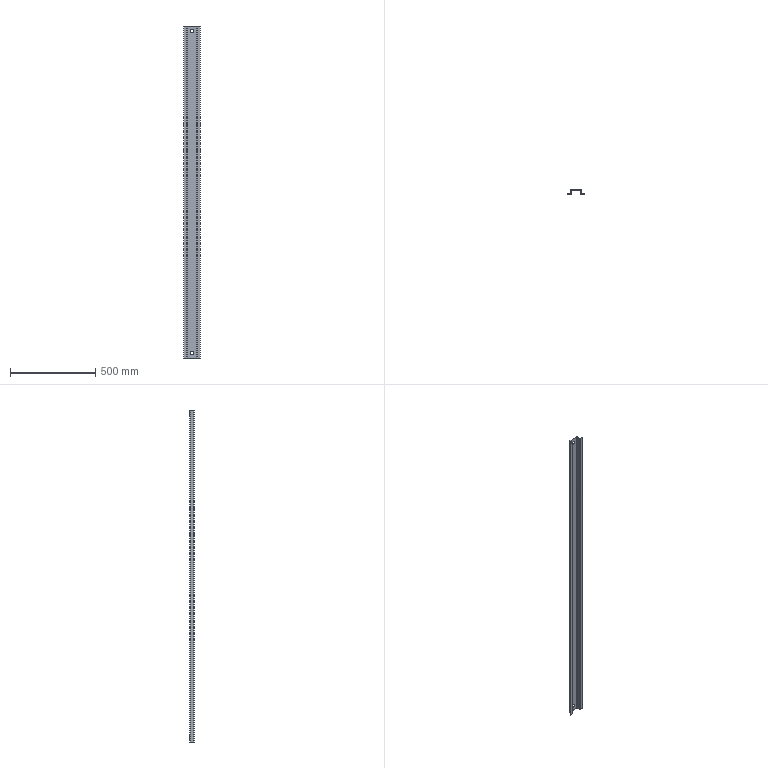Part | 1 solid | 42 faces | box 98.4 x 25 x 1951 mm | volume 224871 mm3 | plane 30 | cylinder 12 | commonest cylinder face diameters 2 x4 3.6 x4 20 x4
STEP:
#1=CARTESIAN_POINT('',(10.,-0.8,945.5));
#2=VERTEX_POINT('',#1);
#3=CARTESIAN_POINT('',(-10.,-0.8,945.5));
#4=VERTEX_POINT('',#3);
#5=CARTESIAN_POINT('',(0.,-0.8,945.5));
#6=DIRECTION('',(0.,1.,0.));
#7=DIRECTION('',(-1.,0.,0.));
#8=AXIS2_PLACEMENT_3D('',#5,#6,#7);
#9=CIRCLE('',#8,10.);
#10=EDGE_CURVE('',#2,#4,#9,.T.);
#11=ORIENTED_EDGE('',*,*,#10,.F.);
#12=CARTESIAN_POINT('',(10.,0.,945.5));
#13=VERTEX_POINT('',#12);
#14=CARTESIAN_POINT('',(10.,-10.,945.5));
#15=DIRECTION('',(0.,1.,0.));
#16=VECTOR('',#15,1000.);
#17=LINE('',#14,#16);
#18=EDGE_CURVE('',#2,#13,#17,.T.);
#19=ORIENTED_EDGE('',*,*,#18,.T.);
#20=CARTESIAN_POINT('',(-10.,0.,945.5));
#21=VERTEX_POINT('',#20);
#22=CARTESIAN_POINT('',(0.,0.,945.5));
#23=DIRECTION('',(0.,1.,0.));
#24=DIRECTION('',(-1.,0.,0.));
#25=AXIS2_PLACEMENT_3D('',#22,#23,#24);
#26=CIRCLE('',#25,10.);
#27=EDGE_CURVE('',#13,#21,#26,.T.);
#28=ORIENTED_EDGE('',*,*,#27,.T.);
#29=CARTESIAN_POINT('',(-10.,-10.,945.5));
#30=DIRECTION('',(0.,1.,0.));
#31=VECTOR('',#30,1000.);
#32=LINE('',#29,#31);
#33=EDGE_CURVE('',#4,#21,#32,.T.);
#34=ORIENTED_EDGE('',*,*,#33,.F.);
#35=EDGE_LOOP('',(#11,#19,#28,#34));
#36=FACE_OUTER_BOUND('',#35,.T.);
#37=CARTESIAN_POINT('',(0.,-10.,945.5));
#38=DIRECTION('',(0.,1.,0.));
#39=DIRECTION('',(-1.,0.,0.));
#40=AXIS2_PLACEMENT_3D('',#37,#38,#39);
#41=CYLINDRICAL_SURFACE('',#40,10.);
#42=ADVANCED_FACE('',(#36),#41,.F.);
#43=CARTESIAN_POINT('',(10.,-0.8,-945.5));
#44=VERTEX_POINT('',#43);
#45=CARTESIAN_POINT('',(-10.,-0.8,-945.5));
#46=VERTEX_POINT('',#45);
#47=CARTESIAN_POINT('',(0.,-0.8,-945.5));
#48=DIRECTION('',(0.,1.,0.));
#49=DIRECTION('',(-1.,0.,0.));
#50=AXIS2_PLACEMENT_3D('',#47,#48,#49);
#51=CIRCLE('',#50,10.);
#52=EDGE_CURVE('',#44,#46,#51,.T.);
#53=ORIENTED_EDGE('',*,*,#52,.F.);
#54=CARTESIAN_POINT('',(10.,0.,-945.5));
#55=VERTEX_POINT('',#54);
#56=CARTESIAN_POINT('',(10.,-10.,-945.5));
#57=DIRECTION('',(0.,1.,0.));
#58=VECTOR('',#57,1000.);
#59=LINE('',#56,#58);
#60=EDGE_CURVE('',#44,#55,#59,.T.);
#61=ORIENTED_EDGE('',*,*,#60,.T.);
#62=CARTESIAN_POINT('',(-10.,0.,-945.5));
#63=VERTEX_POINT('',#62);
#64=CARTESIAN_POINT('',(0.,0.,-945.5));
#65=DIRECTION('',(0.,1.,0.));
#66=DIRECTION('',(1.,0.,0.));
#67=AXIS2_PLACEMENT_3D('',#64,#65,#66);
#68=CIRCLE('',#67,10.);
#69=EDGE_CURVE('',#55,#63,#68,.T.);
#70=ORIENTED_EDGE('',*,*,#69,.T.);
#71=CARTESIAN_POINT('',(-10.,-10.,-945.5));
#72=DIRECTION('',(0.,1.,0.));
#73=VECTOR('',#72,1000.);
#74=LINE('',#71,#73);
#75=EDGE_CURVE('',#46,#63,#74,.T.);
#76=ORIENTED_EDGE('',*,*,#75,.F.);
#77=EDGE_LOOP('',(#53,#61,#70,#76));
#78=FACE_OUTER_BOUND('',#77,.T.);
#79=CARTESIAN_POINT('',(0.,-10.,-945.5));
#80=DIRECTION('',(0.,1.,0.));
#81=DIRECTION('',(-1.,0.,0.));
#82=AXIS2_PLACEMENT_3D('',#79,#80,#81);
#83=CYLINDRICAL_SURFACE('',#82,10.);
#84=ADVANCED_FACE('',(#78),#83,.F.);
#85=CARTESIAN_POINT('',(29.2,-23.2,-975.5));
#86=VERTEX_POINT('',#85);
#87=CARTESIAN_POINT('',(29.2,-23.2,975.5));
#88=VERTEX_POINT('',#87);
#89=CARTESIAN_POINT('',(29.2,-23.2,-975.5));
#90=DIRECTION('',(0.,0.,1.));
#91=VECTOR('',#90,1000.);
#92=LINE('',#89,#91);
#93=EDGE_CURVE('',#86,#88,#92,.T.);
#94=ORIENTED_EDGE('',*,*,#93,.T.);
#95=CARTESIAN_POINT('',(29.2,-1.8,975.5));
#96=VERTEX_POINT('',#95);
#97=CARTESIAN_POINT('',(29.2,0.,975.5));
#98=DIRECTION('',(0.,-1.,0.));
#99=VECTOR('',#98,1000.);
#100=LINE('',#97,#99);
#101=EDGE_CURVE('',#96,#88,#100,.T.);
#102=ORIENTED_EDGE('',*,*,#101,.F.);
#103=CARTESIAN_POINT('',(29.2,-1.8,-975.5));
#104=VERTEX_POINT('',#103);
#105=CARTESIAN_POINT('',(29.2,-1.8,975.5));
#106=DIRECTION('',(0.,0.,-1.));
#107=VECTOR('',#106,1000.);
#108=LINE('',#105,#107);
#109=EDGE_CURVE('',#96,#104,#108,.T.);
#110=ORIENTED_EDGE('',*,*,#109,.T.);
#111=CARTESIAN_POINT('',(29.2,0.,-975.5));
#112=DIRECTION('',(0.,-1.,0.));
#113=VECTOR('',#112,1000.);
#114=LINE('',#111,#113);
#115=EDGE_CURVE('',#104,#86,#114,.T.);
#116=ORIENTED_EDGE('',*,*,#115,.T.);
#117=EDGE_LOOP('',(#94,#102,#110,#116));
#118=FACE_OUTER_BOUND('',#117,.T.);
#119=CARTESIAN_POINT('',(29.2,0.,975.5));
#120=DIRECTION('',(1.,0.,0.));
#121=DIRECTION('',(0.,1.,0.));
#122=AXIS2_PLACEMENT_3D('',#119,#120,#121);
#123=PLANE('',#122);
#124=ADVANCED_FACE('',(#118),#123,.F.);
#125=CARTESIAN_POINT('',(30.,-1.8,975.5));
#126=VERTEX_POINT('',#125);
#127=CARTESIAN_POINT('',(30.,-23.2,975.5));
#128=VERTEX_POINT('',#127);
#129=CARTESIAN_POINT('',(30.,0.,975.5));
#130=DIRECTION('',(0.,-1.,0.));
#131=VECTOR('',#130,1000.);
#132=LINE('',#129,#131);
#133=EDGE_CURVE('',#126,#128,#132,.T.);
#134=ORIENTED_EDGE('',*,*,#133,.T.);
#135=CARTESIAN_POINT('',(30.,-23.2,-975.5));
#136=VERTEX_POINT('',#135);
#137=CARTESIAN_POINT('',(30.,-23.2,-975.5));
#138=DIRECTION('',(0.,0.,1.));
#139=VECTOR('',#138,1000.);
#140=LINE('',#137,#139);
#141=EDGE_CURVE('',#136,#128,#140,.T.);
#142=ORIENTED_EDGE('',*,*,#141,.F.);
#143=CARTESIAN_POINT('',(30.,-1.8,-975.5));
#144=VERTEX_POINT('',#143);
#145=CARTESIAN_POINT('',(30.,0.,-975.5));
#146=DIRECTION('',(0.,-1.,0.));
#147=VECTOR('',#146,1000.);
#148=LINE('',#145,#147);
#149=EDGE_CURVE('',#144,#136,#148,.T.);
#150=ORIENTED_EDGE('',*,*,#149,.F.);
#151=CARTESIAN_POINT('',(30.,-1.8,975.5));
#152=DIRECTION('',(0.,0.,-1.));
#153=VECTOR('',#152,1000.);
#154=LINE('',#151,#153);
#155=EDGE_CURVE('',#126,#144,#154,.T.);
#156=ORIENTED_EDGE('',*,*,#155,.F.);
#157=EDGE_LOOP('',(#134,#142,#150,#156));
#158=FACE_OUTER_BOUND('',#157,.T.);
#159=CARTESIAN_POINT('',(30.,0.,975.5));
#160=DIRECTION('',(1.,0.,0.));
#161=DIRECTION('',(0.,1.,0.));
#162=AXIS2_PLACEMENT_3D('',#159,#160,#161);
#163=PLANE('',#162);
#164=ADVANCED_FACE('',(#158),#163,.T.);
#165=CARTESIAN_POINT('',(30.,-23.2,-975.5));
#166=DIRECTION('',(-1.,0.,0.));
#167=VECTOR('',#166,1000.);
#168=LINE('',#165,#167);
#169=EDGE_CURVE('',#136,#86,#168,.T.);
#170=ORIENTED_EDGE('',*,*,#169,.T.);
#171=ORIENTED_EDGE('',*,*,#115,.F.);
#172=CARTESIAN_POINT('',(29.2,-1.8,-975.5));
#173=DIRECTION('',(1.,0.,0.));
#174=VECTOR('',#173,1000.);
#175=LINE('',#172,#174);
#176=EDGE_CURVE('',#104,#144,#175,.T.);
#177=ORIENTED_EDGE('',*,*,#176,.T.);
#178=ORIENTED_EDGE('',*,*,#149,.T.);
#179=EDGE_LOOP('',(#170,#171,#177,#178));
#180=FACE_OUTER_BOUND('',#179,.T.);
#181=CARTESIAN_POINT('',(28.2,-1.8,-975.5));
#182=DIRECTION('',(0.,0.,1.));
#183=DIRECTION('',(1.,0.,0.));
#184=AXIS2_PLACEMENT_3D('',#181,#182,#183);
#185=PLANE('',#184);
#186=ADVANCED_FACE('',(#180),#185,.F.);
#187=CARTESIAN_POINT('',(-30.,-23.2,-975.5));
#188=VERTEX_POINT('',#187);
#189=CARTESIAN_POINT('',(-30.,-1.8,-975.5));
#190=VERTEX_POINT('',#189);
#191=CARTESIAN_POINT('',(-30.,-25.,-975.5));
#192=DIRECTION('',(0.,1.,0.));
#193=VECTOR('',#192,1000.);
#194=LINE('',#191,#193);
#195=EDGE_CURVE('',#188,#190,#194,.T.);
#196=ORIENTED_EDGE('',*,*,#195,.F.);
#197=CARTESIAN_POINT('',(-30.,-23.2,975.5));
#198=VERTEX_POINT('',#197);
#199=CARTESIAN_POINT('',(-30.,-23.2,975.5));
#200=DIRECTION('',(0.,0.,-1.));
#201=VECTOR('',#200,1000.);
#202=LINE('',#199,#201);
#203=EDGE_CURVE('',#198,#188,#202,.T.);
#204=ORIENTED_EDGE('',*,*,#203,.F.);
#205=CARTESIAN_POINT('',(-30.,-1.8,975.5));
#206=VERTEX_POINT('',#205);
#207=CARTESIAN_POINT('',(-30.,-25.,975.5));
#208=DIRECTION('',(0.,1.,0.));
#209=VECTOR('',#208,1000.);
#210=LINE('',#207,#209);
#211=EDGE_CURVE('',#198,#206,#210,.T.);
#212=ORIENTED_EDGE('',*,*,#211,.T.);
#213=CARTESIAN_POINT('',(-30.,-1.8,975.5));
#214=DIRECTION('',(0.,0.,-1.));
#215=VECTOR('',#214,1000.);
#216=LINE('',#213,#215);
#217=EDGE_CURVE('',#206,#190,#216,.T.);
#218=ORIENTED_EDGE('',*,*,#217,.T.);
#219=EDGE_LOOP('',(#196,#204,#212,#218));
#220=FACE_OUTER_BOUND('',#219,.T.);
#221=CARTESIAN_POINT('',(-30.,-25.,975.5));
#222=DIRECTION('',(-1.,0.,0.));
#223=DIRECTION('',(0.,0.,1.));
#224=AXIS2_PLACEMENT_3D('',#221,#222,#223);
#225=PLANE('',#224);
#226=ADVANCED_FACE('',(#220),#225,.T.);
#227=CARTESIAN_POINT('',(-29.2,-23.2,975.5));
#228=VERTEX_POINT('',#227);
#229=CARTESIAN_POINT('',(-29.2,-23.2,-975.5));
#230=VERTEX_POINT('',#229);
#231=CARTESIAN_POINT('',(-29.2,-23.2,975.5));
#232=DIRECTION('',(0.,0.,-1.));
#233=VECTOR('',#232,1000.);
#234=LINE('',#231,#233);
#235=EDGE_CURVE('',#228,#230,#234,.T.);
#236=ORIENTED_EDGE('',*,*,#235,.T.);
#237=CARTESIAN_POINT('',(-29.2,-1.8,-975.5));
#238=VERTEX_POINT('',#237);
#239=CARTESIAN_POINT('',(-29.2,-25.,-975.5));
#240=DIRECTION('',(0.,1.,0.));
#241=VECTOR('',#240,1000.);
#242=LINE('',#239,#241);
#243=EDGE_CURVE('',#230,#238,#242,.T.);
#244=ORIENTED_EDGE('',*,*,#243,.T.);
#245=CARTESIAN_POINT('',(-29.2,-1.8,975.5));
#246=VERTEX_POINT('',#245);
#247=CARTESIAN_POINT('',(-29.2,-1.8,975.5));
#248=DIRECTION('',(0.,0.,-1.));
#249=VECTOR('',#248,1000.);
#250=LINE('',#247,#249);
#251=EDGE_CURVE('',#246,#238,#250,.T.);
#252=ORIENTED_EDGE('',*,*,#251,.F.);
#253=CARTESIAN_POINT('',(-29.2,-25.,975.5));
#254=DIRECTION('',(0.,1.,0.));
#255=VECTOR('',#254,1000.);
#256=LINE('',#253,#255);
#257=EDGE_CURVE('',#228,#246,#256,.T.);
#258=ORIENTED_EDGE('',*,*,#257,.F.);
#259=EDGE_LOOP('',(#236,#244,#252,#258));
#260=FACE_OUTER_BOUND('',#259,.T.);
#261=CARTESIAN_POINT('',(-29.2,-25.,975.5));
#262=DIRECTION('',(-1.,0.,0.));
#263=DIRECTION('',(0.,0.,1.));
#264=AXIS2_PLACEMENT_3D('',#261,#262,#263);
#265=PLANE('',#264);
#266=ADVANCED_FACE('',(#260),#265,.F.);
#267=ORIENTED_EDGE('',*,*,#211,.F.);
#268=CARTESIAN_POINT('',(-30.,-23.2,975.5));
#269=DIRECTION('',(1.,0.,0.));
#270=VECTOR('',#269,1000.);
#271=LINE('',#268,#270);
#272=EDGE_CURVE('',#198,#228,#271,.T.);
#273=ORIENTED_EDGE('',*,*,#272,.T.);
#274=ORIENTED_EDGE('',*,*,#257,.T.);
#275=CARTESIAN_POINT('',(-29.2,-1.8,975.5));
#276=DIRECTION('',(-1.,0.,0.));
#277=VECTOR('',#276,1000.);
#278=LINE('',#275,#277);
#279=EDGE_CURVE('',#246,#206,#278,.T.);
#280=ORIENTED_EDGE('',*,*,#279,.T.);
#281=EDGE_LOOP('',(#267,#273,#274,#280));
#282=FACE_OUTER_BOUND('',#281,.T.);
#283=CARTESIAN_POINT('',(28.2,-1.8,975.5));
#284=DIRECTION('',(0.,0.,1.));
#285=DIRECTION('',(1.,0.,0.));
#286=AXIS2_PLACEMENT_3D('',#283,#284,#285);
#287=PLANE('',#286);
#288=ADVANCED_FACE('',(#282),#287,.T.);
#289=CARTESIAN_POINT('',(-28.2,0.,975.5));
#290=VERTEX_POINT('',#289);
#291=CARTESIAN_POINT('',(-28.2,-0.8,975.5));
#292=VERTEX_POINT('',#291);
#293=CARTESIAN_POINT('',(-28.2,0.,975.5));
#294=DIRECTION('',(0.,-1.,0.));
#295=VECTOR('',#294,1000.);
#296=LINE('',#293,#295);
#297=EDGE_CURVE('',#290,#292,#296,.T.);
#298=ORIENTED_EDGE('',*,*,#297,.F.);
#299=CARTESIAN_POINT('',(-28.2,-1.8,975.5));
#300=DIRECTION('',(0.,0.,-1.));
#301=DIRECTION('',(1.,0.,0.));
#302=AXIS2_PLACEMENT_3D('',#299,#300,#301);
#303=CIRCLE('',#302,1.8);
#304=EDGE_CURVE('',#206,#290,#303,.T.);
#305=ORIENTED_EDGE('',*,*,#304,.F.);
#306=ORIENTED_EDGE('',*,*,#279,.F.);
#307=CARTESIAN_POINT('',(-28.2,-1.8,975.5));
#308=DIRECTION('',(0.,0.,-1.));
#309=DIRECTION('',(1.,0.,0.));
#310=AXIS2_PLACEMENT_3D('',#307,#308,#309);
#311=CIRCLE('',#310,1.);
#312=EDGE_CURVE('',#246,#292,#311,.T.);
#313=ORIENTED_EDGE('',*,*,#312,.T.);
#314=EDGE_LOOP('',(#298,#305,#306,#313));
#315=FACE_OUTER_BOUND('',#314,.T.);
#316=CARTESIAN_POINT('',(-28.2,0.,975.5));
#317=DIRECTION('',(0.,0.,1.));
#318=DIRECTION('',(1.,0.,0.));
#319=AXIS2_PLACEMENT_3D('',#316,#317,#318);
#320=PLANE('',#319);
#321=ADVANCED_FACE('',(#315),#320,.T.);
#322=CARTESIAN_POINT('',(28.2,0.,975.5));
#323=VERTEX_POINT('',#322);
#324=CARTESIAN_POINT('',(-30.,0.,975.5));
#325=DIRECTION('',(1.,0.,0.));
#326=VECTOR('',#325,1000.);
#327=LINE('',#324,#326);
#328=EDGE_CURVE('',#290,#323,#327,.T.);
#329=ORIENTED_EDGE('',*,*,#328,.F.);
#330=ORIENTED_EDGE('',*,*,#297,.T.);
#331=CARTESIAN_POINT('',(28.2,-0.8,975.5));
#332=VERTEX_POINT('',#331);
#333=CARTESIAN_POINT('',(-30.,-0.8,975.5));
#334=DIRECTION('',(1.,0.,0.));
#335=VECTOR('',#334,1000.);
#336=LINE('',#333,#335);
#337=EDGE_CURVE('',#292,#332,#336,.T.);
#338=ORIENTED_EDGE('',*,*,#337,.T.);
#339=CARTESIAN_POINT('',(28.2,-0.8,975.5));
#340=DIRECTION('',(0.,1.,0.));
#341=VECTOR('',#340,1000.);
#342=LINE('',#339,#341);
#343=EDGE_CURVE('',#332,#323,#342,.T.);
#344=ORIENTED_EDGE('',*,*,#343,.T.);
#345=EDGE_LOOP('',(#329,#330,#338,#344));
#346=FACE_OUTER_BOUND('',#345,.T.);
#347=CARTESIAN_POINT('',(-29.2,-1.8,975.5));
#348=DIRECTION('',(0.,0.,1.));
#349=DIRECTION('',(1.,0.,0.));
#350=AXIS2_PLACEMENT_3D('',#347,#348,#349);
#351=PLANE('',#350);
#352=ADVANCED_FACE('',(#346),#351,.T.);
#353=CARTESIAN_POINT('',(-30.,-1.8,-975.5));
#354=DIRECTION('',(1.,0.,0.));
#355=VECTOR('',#354,1000.);
#356=LINE('',#353,#355);
#357=EDGE_CURVE('',#190,#238,#356,.T.);
#358=ORIENTED_EDGE('',*,*,#357,.F.);
#359=CARTESIAN_POINT('',(-28.2,0.,-975.5));
#360=VERTEX_POINT('',#359);
#361=CARTESIAN_POINT('',(-28.2,-1.8,-975.5));
#362=DIRECTION('',(0.,0.,-1.));
#363=DIRECTION('',(1.,0.,0.));
#364=AXIS2_PLACEMENT_3D('',#361,#362,#363);
#365=CIRCLE('',#364,1.8);
#366=EDGE_CURVE('',#190,#360,#365,.T.);
#367=ORIENTED_EDGE('',*,*,#366,.T.);
#368=CARTESIAN_POINT('',(-28.2,-0.8,-975.5));
#369=VERTEX_POINT('',#368);
#370=CARTESIAN_POINT('',(-28.2,-0.8,-975.5));
#371=DIRECTION('',(0.,1.,0.));
#372=VECTOR('',#371,1000.);
#373=LINE('',#370,#372);
#374=EDGE_CURVE('',#369,#360,#373,.T.);
#375=ORIENTED_EDGE('',*,*,#374,.F.);
#376=CARTESIAN_POINT('',(-28.2,-1.8,-975.5));
#377=DIRECTION('',(0.,0.,-1.));
#378=DIRECTION('',(1.,0.,0.));
#379=AXIS2_PLACEMENT_3D('',#376,#377,#378);
#380=CIRCLE('',#379,1.);
#381=EDGE_CURVE('',#238,#369,#380,.T.);
#382=ORIENTED_EDGE('',*,*,#381,.F.);
#383=EDGE_LOOP('',(#358,#367,#375,#382));
#384=FACE_OUTER_BOUND('',#383,.T.);
#385=CARTESIAN_POINT('',(-30.,-1.8,-975.5));
#386=DIRECTION('',(0.,0.,-1.));
#387=DIRECTION('',(-1.,0.,0.));
#388=AXIS2_PLACEMENT_3D('',#385,#386,#387);
#389=PLANE('',#388);
#390=ADVANCED_FACE('',(#384),#389,.T.);
#391=CARTESIAN_POINT('',(-30.,-23.2,-975.5));
#392=DIRECTION('',(1.,0.,0.));
#393=VECTOR('',#392,1000.);
#394=LINE('',#391,#393);
#395=EDGE_CURVE('',#188,#230,#394,.T.);
#396=ORIENTED_EDGE('',*,*,#395,.F.);
#397=ORIENTED_EDGE('',*,*,#195,.T.);
#398=ORIENTED_EDGE('',*,*,#357,.T.);
#399=ORIENTED_EDGE('',*,*,#243,.F.);
#400=EDGE_LOOP('',(#396,#397,#398,#399));
#401=FACE_OUTER_BOUND('',#400,.T.);
#402=CARTESIAN_POINT('',(-28.2,-0.8,-975.5));
#403=DIRECTION('',(0.,0.,-1.));
#404=DIRECTION('',(-1.,0.,0.));
#405=AXIS2_PLACEMENT_3D('',#402,#403,#404);
#406=PLANE('',#405);
#407=ADVANCED_FACE('',(#401),#406,.T.);
#408=CARTESIAN_POINT('',(30.,-1.8,975.5));
#409=DIRECTION('',(-1.,0.,0.));
#410=VECTOR('',#409,1000.);
#411=LINE('',#408,#410);
#412=EDGE_CURVE('',#126,#96,#411,.T.);
#413=ORIENTED_EDGE('',*,*,#412,.F.);
#414=CARTESIAN_POINT('',(28.2,-1.8,975.5));
#415=DIRECTION('',(0.,0.,-1.));
#416=DIRECTION('',(1.,0.,0.));
#417=AXIS2_PLACEMENT_3D('',#414,#415,#416);
#418=CIRCLE('',#417,1.8);
#419=EDGE_CURVE('',#323,#126,#418,.T.);
#420=ORIENTED_EDGE('',*,*,#419,.F.);
#421=ORIENTED_EDGE('',*,*,#343,.F.);
#422=CARTESIAN_POINT('',(28.2,-1.8,975.5));
#423=DIRECTION('',(0.,0.,-1.));
#424=DIRECTION('',(1.,0.,0.));
#425=AXIS2_PLACEMENT_3D('',#422,#423,#424);
#426=CIRCLE('',#425,1.);
#427=EDGE_CURVE('',#332,#96,#426,.T.);
#428=ORIENTED_EDGE('',*,*,#427,.T.);
#429=EDGE_LOOP('',(#413,#420,#421,#428));
#430=FACE_OUTER_BOUND('',#429,.T.);
#431=CARTESIAN_POINT('',(30.,-1.8,975.5));
#432=DIRECTION('',(0.,0.,1.));
#433=DIRECTION('',(1.,0.,0.));
#434=AXIS2_PLACEMENT_3D('',#431,#432,#433);
#435=PLANE('',#434);
#436=ADVANCED_FACE('',(#430),#435,.T.);
#437=CARTESIAN_POINT('',(30.,-23.2,975.5));
#438=DIRECTION('',(-1.,0.,0.));
#439=VECTOR('',#438,1000.);
#440=LINE('',#437,#439);
#441=EDGE_CURVE('',#128,#88,#440,.T.);
#442=ORIENTED_EDGE('',*,*,#441,.F.);
#443=ORIENTED_EDGE('',*,*,#133,.F.);
#444=ORIENTED_EDGE('',*,*,#412,.T.);
#445=ORIENTED_EDGE('',*,*,#101,.T.);
#446=EDGE_LOOP('',(#442,#443,#444,#445));
#447=FACE_OUTER_BOUND('',#446,.T.);
#448=CARTESIAN_POINT('',(28.2,-0.8,975.5));
#449=DIRECTION('',(0.,0.,1.));
#450=DIRECTION('',(1.,0.,0.));
#451=AXIS2_PLACEMENT_3D('',#448,#449,#450);
#452=PLANE('',#451);
#453=ADVANCED_FACE('',(#447),#452,.T.);
#454=CARTESIAN_POINT('',(28.2,0.,-975.5));
#455=VERTEX_POINT('',#454);
#456=CARTESIAN_POINT('',(28.2,-0.8,-975.5));
#457=VERTEX_POINT('',#456);
#458=CARTESIAN_POINT('',(28.2,0.,-975.5));
#459=DIRECTION('',(0.,-1.,0.));
#460=VECTOR('',#459,1000.);
#461=LINE('',#458,#460);
#462=EDGE_CURVE('',#455,#457,#461,.T.);
#463=ORIENTED_EDGE('',*,*,#462,.F.);
#464=CARTESIAN_POINT('',(28.2,-1.8,-975.5));
#465=DIRECTION('',(0.,0.,-1.));
#466=DIRECTION('',(1.,0.,0.));
#467=AXIS2_PLACEMENT_3D('',#464,#465,#466);
#468=CIRCLE('',#467,1.8);
#469=EDGE_CURVE('',#455,#144,#468,.T.);
#470=ORIENTED_EDGE('',*,*,#469,.T.);
#471=ORIENTED_EDGE('',*,*,#176,.F.);
#472=CARTESIAN_POINT('',(28.2,-1.8,-975.5));
#473=DIRECTION('',(0.,0.,-1.));
#474=DIRECTION('',(1.,0.,0.));
#475=AXIS2_PLACEMENT_3D('',#472,#473,#474);
#476=CIRCLE('',#475,1.);
#477=EDGE_CURVE('',#457,#104,#476,.T.);
#478=ORIENTED_EDGE('',*,*,#477,.F.);
#479=EDGE_LOOP('',(#463,#470,#471,#478));
#480=FACE_OUTER_BOUND('',#479,.T.);
#481=CARTESIAN_POINT('',(28.2,0.,-975.5));
#482=DIRECTION('',(0.,0.,-1.));
#483=DIRECTION('',(-1.,0.,0.));
#484=AXIS2_PLACEMENT_3D('',#481,#482,#483);
#485=PLANE('',#484);
#486=ADVANCED_FACE('',(#480),#485,.T.);
#487=CARTESIAN_POINT('',(-30.,0.,-975.5));
#488=DIRECTION('',(1.,0.,0.));
#489=VECTOR('',#488,1000.);
#490=LINE('',#487,#489);
#491=EDGE_CURVE('',#360,#455,#490,.T.);
#492=ORIENTED_EDGE('',*,*,#491,.T.);
#493=ORIENTED_EDGE('',*,*,#462,.T.);
#494=CARTESIAN_POINT('',(-30.,-0.8,-975.5));
#495=DIRECTION('',(1.,0.,0.));
#496=VECTOR('',#495,1000.);
#497=LINE('',#494,#496);
#498=EDGE_CURVE('',#369,#457,#497,.T.);
#499=ORIENTED_EDGE('',*,*,#498,.F.);
#500=ORIENTED_EDGE('',*,*,#374,.T.);
#501=EDGE_LOOP('',(#492,#493,#499,#500));
#502=FACE_OUTER_BOUND('',#501,.T.);
#503=CARTESIAN_POINT('',(29.2,-1.8,-975.5));
#504=DIRECTION('',(0.,0.,-1.));
#505=DIRECTION('',(-1.,0.,0.));
#506=AXIS2_PLACEMENT_3D('',#503,#504,#505);
#507=PLANE('',#506);
#508=ADVANCED_FACE('',(#502),#507,.T.);
#509=ORIENTED_EDGE('',*,*,#469,.F.);
#510=CARTESIAN_POINT('',(28.2,0.,975.5));
#511=DIRECTION('',(0.,0.,-1.));
#512=VECTOR('',#511,1000.);
#513=LINE('',#510,#512);
#514=EDGE_CURVE('',#323,#455,#513,.T.);
#515=ORIENTED_EDGE('',*,*,#514,.F.);
#516=ORIENTED_EDGE('',*,*,#419,.T.);
#517=ORIENTED_EDGE('',*,*,#155,.T.);
#518=EDGE_LOOP('',(#509,#515,#516,#517));
#519=FACE_OUTER_BOUND('',#518,.T.);
#520=CARTESIAN_POINT('',(28.2,-1.8,975.5));
#521=DIRECTION('',(0.,0.,-1.));
#522=DIRECTION('',(-1.,0.,0.));
#523=AXIS2_PLACEMENT_3D('',#520,#521,#522);
#524=CYLINDRICAL_SURFACE('',#523,1.8);
#525=ADVANCED_FACE('',(#519),#524,.T.);
#526=CARTESIAN_POINT('',(0.,0.,945.5));
#527=DIRECTION('',(0.,1.,0.));
#528=DIRECTION('',(-1.,0.,0.));
#529=AXIS2_PLACEMENT_3D('',#526,#527,#528);
#530=CIRCLE('',#529,10.);
#531=EDGE_CURVE('',#21,#13,#530,.T.);
#532=ORIENTED_EDGE('',*,*,#531,.F.);
#533=ORIENTED_EDGE('',*,*,#27,.F.);
#534=EDGE_LOOP('',(#532,#533));
#535=FACE_BOUND('',#534,.T.);
#536=CARTESIAN_POINT('',(0.,0.,-945.5));
#537=DIRECTION('',(0.,1.,0.));
#538=DIRECTION('',(1.,0.,0.));
#539=AXIS2_PLACEMENT_3D('',#536,#537,#538);
#540=CIRCLE('',#539,10.);
#541=EDGE_CURVE('',#63,#55,#540,.T.);
#542=ORIENTED_EDGE('',*,*,#541,.F.);
#543=ORIENTED_EDGE('',*,*,#69,.F.);
#544=EDGE_LOOP('',(#542,#543));
#545=FACE_BOUND('',#544,.T.);
#546=ORIENTED_EDGE('',*,*,#491,.F.);
#547=CARTESIAN_POINT('',(-28.2,0.,975.5));
#548=DIRECTION('',(0.,0.,-1.));
#549=VECTOR('',#548,1000.);
#550=LINE('',#547,#549);
#551=EDGE_CURVE('',#290,#360,#550,.T.);
#552=ORIENTED_EDGE('',*,*,#551,.F.);
#553=ORIENTED_EDGE('',*,*,#328,.T.);
#554=ORIENTED_EDGE('',*,*,#514,.T.);
#555=EDGE_LOOP('',(#546,#552,#553,#554));
#556=FACE_OUTER_BOUND('',#555,.T.);
#557=CARTESIAN_POINT('',(-30.,0.,975.5));
#558=DIRECTION('',(0.,1.,0.));
#559=DIRECTION('',(-1.,0.,0.));
#560=AXIS2_PLACEMENT_3D('',#557,#558,#559);
#561=PLANE('',#560);
#562=ADVANCED_FACE('',(#535,#545,#556),#561,.T.);
#563=ORIENTED_EDGE('',*,*,#366,.F.);
#564=ORIENTED_EDGE('',*,*,#217,.F.);
#565=ORIENTED_EDGE('',*,*,#304,.T.);
#566=ORIENTED_EDGE('',*,*,#551,.T.);
#567=EDGE_LOOP('',(#563,#564,#565,#566));
#568=FACE_OUTER_BOUND('',#567,.T.);
#569=CARTESIAN_POINT('',(-28.2,-1.8,975.5));
#570=DIRECTION('',(0.,0.,-1.));
#571=DIRECTION('',(-1.,0.,0.));
#572=AXIS2_PLACEMENT_3D('',#569,#570,#571);
#573=CYLINDRICAL_SURFACE('',#572,1.8);
#574=ADVANCED_FACE('',(#568),#573,.T.);
#575=ORIENTED_EDGE('',*,*,#381,.T.);
#576=CARTESIAN_POINT('',(-28.2,-0.8,975.5));
#577=DIRECTION('',(0.,0.,-1.));
#578=VECTOR('',#577,1000.);
#579=LINE('',#576,#578);
#580=EDGE_CURVE('',#292,#369,#579,.T.);
#581=ORIENTED_EDGE('',*,*,#580,.F.);
#582=ORIENTED_EDGE('',*,*,#312,.F.);
#583=ORIENTED_EDGE('',*,*,#251,.T.);
#584=EDGE_LOOP('',(#575,#581,#582,#583));
#585=FACE_OUTER_BOUND('',#584,.T.);
#586=CARTESIAN_POINT('',(-28.2,-1.8,975.5));
#587=DIRECTION('',(0.,0.,-1.));
#588=DIRECTION('',(-1.,0.,0.));
#589=AXIS2_PLACEMENT_3D('',#586,#587,#588);
#590=CYLINDRICAL_SURFACE('',#589,1.);
#591=ADVANCED_FACE('',(#585),#590,.F.);
#592=CARTESIAN_POINT('',(0.,-0.8,945.5));
#593=DIRECTION('',(0.,1.,0.));
#594=DIRECTION('',(-1.,0.,0.));
#595=AXIS2_PLACEMENT_3D('',#592,#593,#594);
#596=CIRCLE('',#595,10.);
#597=EDGE_CURVE('',#4,#2,#596,.T.);
#598=ORIENTED_EDGE('',*,*,#597,.T.);
#599=ORIENTED_EDGE('',*,*,#10,.T.);
#600=EDGE_LOOP('',(#598,#599));
#601=FACE_BOUND('',#600,.T.);
#602=CARTESIAN_POINT('',(0.,-0.8,-945.5));
#603=DIRECTION('',(0.,1.,0.));
#604=DIRECTION('',(-1.,0.,0.));
#605=AXIS2_PLACEMENT_3D('',#602,#603,#604);
#606=CIRCLE('',#605,10.);
#607=EDGE_CURVE('',#46,#44,#606,.T.);
#608=ORIENTED_EDGE('',*,*,#607,.T.);
#609=ORIENTED_EDGE('',*,*,#52,.T.);
#610=EDGE_LOOP('',(#608,#609));
#611=FACE_BOUND('',#610,.T.);
#612=ORIENTED_EDGE('',*,*,#498,.T.);
#613=CARTESIAN_POINT('',(28.2,-0.8,975.5));
#614=DIRECTION('',(0.,0.,-1.));
#615=VECTOR('',#614,1000.);
#616=LINE('',#613,#615);
#617=EDGE_CURVE('',#332,#457,#616,.T.);
#618=ORIENTED_EDGE('',*,*,#617,.F.);
#619=ORIENTED_EDGE('',*,*,#337,.F.);
#620=ORIENTED_EDGE('',*,*,#580,.T.);
#621=EDGE_LOOP('',(#612,#618,#619,#620));
#622=FACE_OUTER_BOUND('',#621,.T.);
#623=CARTESIAN_POINT('',(-30.,-0.8,975.5));
#624=DIRECTION('',(0.,1.,0.));
#625=DIRECTION('',(-1.,0.,0.));
#626=AXIS2_PLACEMENT_3D('',#623,#624,#625);
#627=PLANE('',#626);
#628=ADVANCED_FACE('',(#601,#611,#622),#627,.F.);
#629=ORIENTED_EDGE('',*,*,#477,.T.);
#630=ORIENTED_EDGE('',*,*,#109,.F.);
#631=ORIENTED_EDGE('',*,*,#427,.F.);
#632=ORIENTED_EDGE('',*,*,#617,.T.);
#633=EDGE_LOOP('',(#629,#630,#631,#632));
#634=FACE_OUTER_BOUND('',#633,.T.);
#635=CARTESIAN_POINT('',(28.2,-1.8,975.5));
#636=DIRECTION('',(0.,0.,-1.));
#637=DIRECTION('',(-1.,0.,0.));
#638=AXIS2_PLACEMENT_3D('',#635,#636,#637);
#639=CYLINDRICAL_SURFACE('',#638,1.);
#640=ADVANCED_FACE('',(#634),#639,.F.);
#641=CARTESIAN_POINT('',(-31.,-24.2,-975.5));
#642=VERTEX_POINT('',#641);
#643=CARTESIAN_POINT('',(-31.,-25.,-975.5));
#644=VERTEX_POINT('',#643);
#645=CARTESIAN_POINT('',(-31.,-25.,-975.5));
#646=DIRECTION('',(0.,-1.,0.));
#647=VECTOR('',#646,1000.);
#648=LINE('',#645,#647);
#649=EDGE_CURVE('',#642,#644,#648,.T.);
#650=ORIENTED_EDGE('',*,*,#649,.F.);
#651=CARTESIAN_POINT('',(-31.,-23.2,-975.5));
#652=DIRECTION('',(0.,0.,-1.));
#653=DIRECTION('',(1.,0.,0.));
#654=AXIS2_PLACEMENT_3D('',#651,#652,#653);
#655=CIRCLE('',#654,1.);
#656=EDGE_CURVE('',#188,#642,#655,.T.);
#657=ORIENTED_EDGE('',*,*,#656,.F.);
#658=ORIENTED_EDGE('',*,*,#395,.T.);
#659=CARTESIAN_POINT('',(-31.,-23.2,-975.5));
#660=DIRECTION('',(0.,0.,-1.));
#661=DIRECTION('',(1.,0.,0.));
#662=AXIS2_PLACEMENT_3D('',#659,#660,#661);
#663=CIRCLE('',#662,1.8);
#664=EDGE_CURVE('',#230,#644,#663,.T.);
#665=ORIENTED_EDGE('',*,*,#664,.T.);
#666=EDGE_LOOP('',(#650,#657,#658,#665));
#667=FACE_OUTER_BOUND('',#666,.T.);
#668=CARTESIAN_POINT('',(-31.,-23.2,-975.5));
#669=DIRECTION('',(0.,0.,-1.));
#670=DIRECTION('',(-1.,0.,0.));
#671=AXIS2_PLACEMENT_3D('',#668,#669,#670);
#672=PLANE('',#671);
#673=ADVANCED_FACE('',(#667),#672,.T.);
#674=CARTESIAN_POINT('',(-31.,-24.2,975.5));
#675=VERTEX_POINT('',#674);
#676=CARTESIAN_POINT('',(-31.,-23.2,975.5));
#677=DIRECTION('',(0.,0.,1.));
#678=DIRECTION('',(1.,0.,0.));
#679=AXIS2_PLACEMENT_3D('',#676,#677,#678);
#680=CIRCLE('',#679,1.);
#681=EDGE_CURVE('',#675,#198,#680,.T.);
#682=ORIENTED_EDGE('',*,*,#681,.F.);
#683=CARTESIAN_POINT('',(-31.,-25.,975.5));
#684=VERTEX_POINT('',#683);
#685=CARTESIAN_POINT('',(-31.,-24.2,975.5));
#686=DIRECTION('',(0.,-1.,0.));
#687=VECTOR('',#686,1000.);
#688=LINE('',#685,#687);
#689=EDGE_CURVE('',#675,#684,#688,.T.);
#690=ORIENTED_EDGE('',*,*,#689,.T.);
#691=CARTESIAN_POINT('',(-31.,-23.2,975.5));
#692=DIRECTION('',(0.,0.,1.));
#693=DIRECTION('',(1.,0.,0.));
#694=AXIS2_PLACEMENT_3D('',#691,#692,#693);
#695=CIRCLE('',#694,1.8);
#696=EDGE_CURVE('',#684,#228,#695,.T.);
#697=ORIENTED_EDGE('',*,*,#696,.T.);
#698=ORIENTED_EDGE('',*,*,#272,.F.);
#699=EDGE_LOOP('',(#682,#690,#697,#698));
#700=FACE_OUTER_BOUND('',#699,.T.);
#701=CARTESIAN_POINT('',(-31.,-23.2,975.5));
#702=DIRECTION('',(0.,0.,-1.));
#703=DIRECTION('',(-1.,0.,0.));
#704=AXIS2_PLACEMENT_3D('',#701,#702,#703);
#705=PLANE('',#704);
#706=ADVANCED_FACE('',(#700),#705,.F.);
#707=ORIENTED_EDGE('',*,*,#235,.F.);
#708=ORIENTED_EDGE('',*,*,#696,.F.);
#709=CARTESIAN_POINT('',(-31.,-25.,-975.5));
#710=DIRECTION('',(0.,0.,-1.));
#711=VECTOR('',#710,1000.);
#712=LINE('',#709,#711);
#713=EDGE_CURVE('',#684,#644,#712,.T.);
#714=ORIENTED_EDGE('',*,*,#713,.T.);
#715=ORIENTED_EDGE('',*,*,#664,.F.);
#716=EDGE_LOOP('',(#707,#708,#714,#715));
#717=FACE_OUTER_BOUND('',#716,.T.);
#718=CARTESIAN_POINT('',(-31.,-23.2,975.5));
#719=DIRECTION('',(0.,0.,1.));
#720=DIRECTION('',(0.,-1.,0.));
#721=AXIS2_PLACEMENT_3D('',#718,#719,#720);
#722=CYLINDRICAL_SURFACE('',#721,1.8);
#723=ADVANCED_FACE('',(#717),#722,.T.);
#724=ORIENTED_EDGE('',*,*,#203,.T.);
#725=ORIENTED_EDGE('',*,*,#656,.T.);
#726=CARTESIAN_POINT('',(-31.,-24.2,-975.5));
#727=DIRECTION('',(0.,0.,1.));
#728=VECTOR('',#727,1000.);
#729=LINE('',#726,#728);
#730=EDGE_CURVE('',#642,#675,#729,.T.);
#731=ORIENTED_EDGE('',*,*,#730,.T.);
#732=ORIENTED_EDGE('',*,*,#681,.T.);
#733=EDGE_LOOP('',(#724,#725,#731,#732));
#734=FACE_OUTER_BOUND('',#733,.T.);
#735=CARTESIAN_POINT('',(-31.,-23.2,975.5));
#736=DIRECTION('',(0.,0.,1.));
#737=DIRECTION('',(0.,-1.,0.));
#738=AXIS2_PLACEMENT_3D('',#735,#736,#737);
#739=CYLINDRICAL_SURFACE('',#738,1.);
#740=ADVANCED_FACE('',(#734),#739,.F.);
#741=ORIENTED_EDGE('',*,*,#689,.F.);
#742=CARTESIAN_POINT('',(-49.2,-24.2,975.5));
#743=VERTEX_POINT('',#742);
#744=CARTESIAN_POINT('',(-49.2,-24.2,975.5));
#745=DIRECTION('',(-1.,0.,0.));
#746=VECTOR('',#745,1000.);
#747=LINE('',#744,#746);
#748=EDGE_CURVE('',#675,#743,#747,.T.);
#749=ORIENTED_EDGE('',*,*,#748,.T.);
#750=CARTESIAN_POINT('',(-49.2,-25.,975.5));
#751=VERTEX_POINT('',#750);
#752=CARTESIAN_POINT('',(-49.2,-25.,975.5));
#753=DIRECTION('',(0.,1.,0.));
#754=VECTOR('',#753,1000.);
#755=LINE('',#752,#754);
#756=EDGE_CURVE('',#751,#743,#755,.T.);
#757=ORIENTED_EDGE('',*,*,#756,.F.);
#758=CARTESIAN_POINT('',(0.,-25.,975.5));
#759=DIRECTION('',(-1.,0.,0.));
#760=VECTOR('',#759,1000.);
#761=LINE('',#758,#760);
#762=EDGE_CURVE('',#684,#751,#761,.T.);
#763=ORIENTED_EDGE('',*,*,#762,.F.);
#764=EDGE_LOOP('',(#741,#749,#757,#763));
#765=FACE_OUTER_BOUND('',#764,.T.);
#766=CARTESIAN_POINT('',(-49.2,-25.,975.5));
#767=DIRECTION('',(0.,0.,-1.));
#768=DIRECTION('',(-1.,0.,0.));
#769=AXIS2_PLACEMENT_3D('',#766,#767,#768);
#770=PLANE('',#769);
#771=ADVANCED_FACE('',(#765),#770,.F.);
#772=ORIENTED_EDGE('',*,*,#649,.T.);
#773=CARTESIAN_POINT('',(-49.2,-25.,-975.5));
#774=VERTEX_POINT('',#773);
#775=CARTESIAN_POINT('',(0.,-25.,-975.5));
#776=DIRECTION('',(1.,0.,0.));
#777=VECTOR('',#776,1000.);
#778=LINE('',#775,#777);
#779=EDGE_CURVE('',#774,#644,#778,.T.);
#780=ORIENTED_EDGE('',*,*,#779,.F.);
#781=CARTESIAN_POINT('',(-49.2,-24.2,-975.5));
#782=VERTEX_POINT('',#781);
#783=CARTESIAN_POINT('',(-49.2,-25.,-975.5));
#784=DIRECTION('',(0.,1.,0.));
#785=VECTOR('',#784,1000.);
#786=LINE('',#783,#785);
#787=EDGE_CURVE('',#774,#782,#786,.T.);
#788=ORIENTED_EDGE('',*,*,#787,.T.);
#789=CARTESIAN_POINT('',(-30.,-24.2,-975.5));
#790=DIRECTION('',(1.,0.,0.));
#791=VECTOR('',#790,1000.);
#792=LINE('',#789,#791);
#793=EDGE_CURVE('',#782,#642,#792,.T.);
#794=ORIENTED_EDGE('',*,*,#793,.T.);
#795=EDGE_LOOP('',(#772,#780,#788,#794));
#796=FACE_OUTER_BOUND('',#795,.T.);
#797=CARTESIAN_POINT('',(-30.,-25.,-975.5));
#798=DIRECTION('',(0.,0.,1.));
#799=DIRECTION('',(1.,0.,0.));
#800=AXIS2_PLACEMENT_3D('',#797,#798,#799);
#801=PLANE('',#800);
#802=ADVANCED_FACE('',(#796),#801,.F.);
#803=ORIENTED_EDGE('',*,*,#713,.F.);
#804=ORIENTED_EDGE('',*,*,#762,.T.);
#805=CARTESIAN_POINT('',(-49.2,-25.,0.));
#806=DIRECTION('',(0.,0.,-1.));
#807=VECTOR('',#806,1000.);
#808=LINE('',#805,#807);
#809=EDGE_CURVE('',#751,#774,#808,.T.);
#810=ORIENTED_EDGE('',*,*,#809,.T.);
#811=ORIENTED_EDGE('',*,*,#779,.T.);
#812=EDGE_LOOP('',(#803,#804,#810,#811));
#813=FACE_OUTER_BOUND('',#812,.T.);
#814=CARTESIAN_POINT('',(0.,-25.,0.));
#815=DIRECTION('',(0.,1.,0.));
#816=DIRECTION('',(-1.,0.,0.));
#817=AXIS2_PLACEMENT_3D('',#814,#815,#816);
#818=PLANE('',#817);
#819=ADVANCED_FACE('',(#813),#818,.F.);
#820=ORIENTED_EDGE('',*,*,#748,.F.);
#821=ORIENTED_EDGE('',*,*,#730,.F.);
#822=ORIENTED_EDGE('',*,*,#793,.F.);
#823=CARTESIAN_POINT('',(-49.2,-24.2,-975.5));
#824=DIRECTION('',(0.,0.,-1.));
#825=VECTOR('',#824,1000.);
#826=LINE('',#823,#825);
#827=EDGE_CURVE('',#743,#782,#826,.T.);
#828=ORIENTED_EDGE('',*,*,#827,.F.);
#829=EDGE_LOOP('',(#820,#821,#822,#828));
#830=FACE_OUTER_BOUND('',#829,.T.);
#831=CARTESIAN_POINT('',(0.,-24.2,0.));
#832=DIRECTION('',(0.,1.,0.));
#833=DIRECTION('',(-1.,0.,0.));
#834=AXIS2_PLACEMENT_3D('',#831,#832,#833);
#835=PLANE('',#834);
#836=ADVANCED_FACE('',(#830),#835,.T.);
#837=ORIENTED_EDGE('',*,*,#827,.T.);
#838=ORIENTED_EDGE('',*,*,#787,.F.);
#839=ORIENTED_EDGE('',*,*,#809,.F.);
#840=ORIENTED_EDGE('',*,*,#756,.T.);
#841=EDGE_LOOP('',(#837,#838,#839,#840));
#842=FACE_OUTER_BOUND('',#841,.T.);
#843=CARTESIAN_POINT('',(-49.2,-25.,-975.5));
#844=DIRECTION('',(1.,0.,0.));
#845=DIRECTION('',(0.,1.,0.));
#846=AXIS2_PLACEMENT_3D('',#843,#844,#845);
#847=PLANE('',#846);
#848=ADVANCED_FACE('',(#842),#847,.F.);
#849=CARTESIAN_POINT('',(31.,-24.2,975.5));
#850=VERTEX_POINT('',#849);
#851=CARTESIAN_POINT('',(31.,-25.,975.5));
#852=VERTEX_POINT('',#851);
#853=CARTESIAN_POINT('',(31.,-25.,975.5));
#854=DIRECTION('',(0.,-1.,0.));
#855=VECTOR('',#854,1000.);
#856=LINE('',#853,#855);
#857=EDGE_CURVE('',#850,#852,#856,.T.);
#858=ORIENTED_EDGE('',*,*,#857,.F.);
#859=CARTESIAN_POINT('',(31.,-23.2,975.5));
#860=DIRECTION('',(0.,0.,1.));
#861=DIRECTION('',(-1.,0.,0.));
#862=AXIS2_PLACEMENT_3D('',#859,#860,#861);
#863=CIRCLE('',#862,1.);
#864=EDGE_CURVE('',#128,#850,#863,.T.);
#865=ORIENTED_EDGE('',*,*,#864,.F.);
#866=ORIENTED_EDGE('',*,*,#441,.T.);
#867=CARTESIAN_POINT('',(31.,-23.2,975.5));
#868=DIRECTION('',(0.,0.,1.));
#869=DIRECTION('',(-1.,0.,0.));
#870=AXIS2_PLACEMENT_3D('',#867,#868,#869);
#871=CIRCLE('',#870,1.8);
#872=EDGE_CURVE('',#88,#852,#871,.T.);
#873=ORIENTED_EDGE('',*,*,#872,.T.);
#874=EDGE_LOOP('',(#858,#865,#866,#873));
#875=FACE_OUTER_BOUND('',#874,.T.);
#876=CARTESIAN_POINT('',(31.,-23.2,975.5));
#877=DIRECTION('',(0.,0.,1.));
#878=DIRECTION('',(1.,0.,0.));
#879=AXIS2_PLACEMENT_3D('',#876,#877,#878);
#880=PLANE('',#879);
#881=ADVANCED_FACE('',(#875),#880,.T.);
#882=CARTESIAN_POINT('',(31.,-24.2,-975.5));
#883=VERTEX_POINT('',#882);
#884=CARTESIAN_POINT('',(31.,-23.2,-975.5));
#885=DIRECTION('',(0.,0.,-1.));
#886=DIRECTION('',(-1.,0.,0.));
#887=AXIS2_PLACEMENT_3D('',#884,#885,#886);
#888=CIRCLE('',#887,1.);
#889=EDGE_CURVE('',#883,#136,#888,.T.);
#890=ORIENTED_EDGE('',*,*,#889,.F.);
#891=CARTESIAN_POINT('',(31.,-25.,-975.5));
#892=VERTEX_POINT('',#891);
#893=CARTESIAN_POINT('',(31.,-24.2,-975.5));
#894=DIRECTION('',(0.,-1.,0.));
#895=VECTOR('',#894,1000.);
#896=LINE('',#893,#895);
#897=EDGE_CURVE('',#883,#892,#896,.T.);
#898=ORIENTED_EDGE('',*,*,#897,.T.);
#899=CARTESIAN_POINT('',(31.,-23.2,-975.5));
#900=DIRECTION('',(0.,0.,-1.));
#901=DIRECTION('',(-1.,0.,0.));
#902=AXIS2_PLACEMENT_3D('',#899,#900,#901);
#903=CIRCLE('',#902,1.8);
#904=EDGE_CURVE('',#892,#86,#903,.T.);
#905=ORIENTED_EDGE('',*,*,#904,.T.);
#906=ORIENTED_EDGE('',*,*,#169,.F.);
#907=EDGE_LOOP('',(#890,#898,#905,#906));
#908=FACE_OUTER_BOUND('',#907,.T.);
#909=CARTESIAN_POINT('',(31.,-23.2,-975.5));
#910=DIRECTION('',(0.,0.,1.));
#911=DIRECTION('',(1.,0.,0.));
#912=AXIS2_PLACEMENT_3D('',#909,#910,#911);
#913=PLANE('',#912);
#914=ADVANCED_FACE('',(#908),#913,.F.);
#915=ORIENTED_EDGE('',*,*,#93,.F.);
#916=ORIENTED_EDGE('',*,*,#904,.F.);
#917=CARTESIAN_POINT('',(31.,-25.,975.5));
#918=DIRECTION('',(0.,0.,1.));
#919=VECTOR('',#918,1000.);
#920=LINE('',#917,#919);
#921=EDGE_CURVE('',#892,#852,#920,.T.);
#922=ORIENTED_EDGE('',*,*,#921,.T.);
#923=ORIENTED_EDGE('',*,*,#872,.F.);
#924=EDGE_LOOP('',(#915,#916,#922,#923));
#925=FACE_OUTER_BOUND('',#924,.T.);
#926=CARTESIAN_POINT('',(31.,-23.2,-975.5));
#927=DIRECTION('',(0.,0.,-1.));
#928=DIRECTION('',(0.,-1.,0.));
#929=AXIS2_PLACEMENT_3D('',#926,#927,#928);
#930=CYLINDRICAL_SURFACE('',#929,1.8);
#931=ADVANCED_FACE('',(#925),#930,.T.);
#932=ORIENTED_EDGE('',*,*,#141,.T.);
#933=ORIENTED_EDGE('',*,*,#864,.T.);
#934=CARTESIAN_POINT('',(31.,-24.2,975.5));
#935=DIRECTION('',(0.,0.,-1.));
#936=VECTOR('',#935,1000.);
#937=LINE('',#934,#936);
#938=EDGE_CURVE('',#850,#883,#937,.T.);
#939=ORIENTED_EDGE('',*,*,#938,.T.);
#940=ORIENTED_EDGE('',*,*,#889,.T.);
#941=EDGE_LOOP('',(#932,#933,#939,#940));
#942=FACE_OUTER_BOUND('',#941,.T.);
#943=CARTESIAN_POINT('',(31.,-23.2,-975.5));
#944=DIRECTION('',(0.,0.,-1.));
#945=DIRECTION('',(0.,-1.,0.));
#946=AXIS2_PLACEMENT_3D('',#943,#944,#945);
#947=CYLINDRICAL_SURFACE('',#946,1.);
#948=ADVANCED_FACE('',(#942),#947,.F.);
#949=ORIENTED_EDGE('',*,*,#857,.T.);
#950=CARTESIAN_POINT('',(49.2,-25.,975.5));
#951=VERTEX_POINT('',#950);
#952=CARTESIAN_POINT('',(0.,-25.,975.5));
#953=DIRECTION('',(-1.,0.,0.));
#954=VECTOR('',#953,1000.);
#955=LINE('',#952,#954);
#956=EDGE_CURVE('',#951,#852,#955,.T.);
#957=ORIENTED_EDGE('',*,*,#956,.F.);
#958=CARTESIAN_POINT('',(49.2,-24.2,975.5));
#959=VERTEX_POINT('',#958);
#960=CARTESIAN_POINT('',(49.2,-25.,975.5));
#961=DIRECTION('',(0.,1.,0.));
#962=VECTOR('',#961,1000.);
#963=LINE('',#960,#962);
#964=EDGE_CURVE('',#951,#959,#963,.T.);
#965=ORIENTED_EDGE('',*,*,#964,.T.);
#966=CARTESIAN_POINT('',(30.,-24.2,975.5));
#967=DIRECTION('',(-1.,0.,0.));
#968=VECTOR('',#967,1000.);
#969=LINE('',#966,#968);
#970=EDGE_CURVE('',#959,#850,#969,.T.);
#971=ORIENTED_EDGE('',*,*,#970,.T.);
#972=EDGE_LOOP('',(#949,#957,#965,#971));
#973=FACE_OUTER_BOUND('',#972,.T.);
#974=CARTESIAN_POINT('',(30.,-25.,975.5));
#975=DIRECTION('',(0.,0.,-1.));
#976=DIRECTION('',(-1.,0.,0.));
#977=AXIS2_PLACEMENT_3D('',#974,#975,#976);
#978=PLANE('',#977);
#979=ADVANCED_FACE('',(#973),#978,.F.);
#980=ORIENTED_EDGE('',*,*,#897,.F.);
#981=CARTESIAN_POINT('',(49.2,-24.2,-975.5));
#982=VERTEX_POINT('',#981);
#983=CARTESIAN_POINT('',(49.2,-24.2,-975.5));
#984=DIRECTION('',(1.,0.,0.));
#985=VECTOR('',#984,1000.);
#986=LINE('',#983,#985);
#987=EDGE_CURVE('',#883,#982,#986,.T.);
#988=ORIENTED_EDGE('',*,*,#987,.T.);
#989=CARTESIAN_POINT('',(49.2,-25.,-975.5));
#990=VERTEX_POINT('',#989);
#991=CARTESIAN_POINT('',(49.2,-25.,-975.5));
#992=DIRECTION('',(0.,1.,0.));
#993=VECTOR('',#992,1000.);
#994=LINE('',#991,#993);
#995=EDGE_CURVE('',#990,#982,#994,.T.);
#996=ORIENTED_EDGE('',*,*,#995,.F.);
#997=CARTESIAN_POINT('',(0.,-25.,-975.5));
#998=DIRECTION('',(1.,0.,0.));
#999=VECTOR('',#998,1000.);
#1000=LINE('',#997,#999);
#1001=EDGE_CURVE('',#892,#990,#1000,.T.);
#1002=ORIENTED_EDGE('',*,*,#1001,.F.);
#1003=EDGE_LOOP('',(#980,#988,#996,#1002));
#1004=FACE_OUTER_BOUND('',#1003,.T.);
#1005=CARTESIAN_POINT('',(49.2,-25.,-975.5));
#1006=DIRECTION('',(0.,0.,1.));
#1007=DIRECTION('',(1.,0.,0.));
#1008=AXIS2_PLACEMENT_3D('',#1005,#1006,#1007);
#1009=PLANE('',#1008);
#1010=ADVANCED_FACE('',(#1004),#1009,.F.);
#1011=ORIENTED_EDGE('',*,*,#921,.F.);
#1012=ORIENTED_EDGE('',*,*,#1001,.T.);
#1013=CARTESIAN_POINT('',(49.2,-25.,0.));
#1014=DIRECTION('',(0.,0.,1.));
#1015=VECTOR('',#1014,1000.);
#1016=LINE('',#1013,#1015);
#1017=EDGE_CURVE('',#990,#951,#1016,.T.);
#1018=ORIENTED_EDGE('',*,*,#1017,.T.);
#1019=ORIENTED_EDGE('',*,*,#956,.T.);
#1020=EDGE_LOOP('',(#1011,#1012,#1018,#1019));
#1021=FACE_OUTER_BOUND('',#1020,.T.);
#1022=CARTESIAN_POINT('',(0.,-25.,0.));
#1023=DIRECTION('',(0.,1.,0.));
#1024=DIRECTION('',(-1.,0.,0.));
#1025=AXIS2_PLACEMENT_3D('',#1022,#1023,#1024);
#1026=PLANE('',#1025);
#1027=ADVANCED_FACE('',(#1021),#1026,.F.);
#1028=ORIENTED_EDGE('',*,*,#987,.F.);
#1029=ORIENTED_EDGE('',*,*,#938,.F.);
#1030=ORIENTED_EDGE('',*,*,#970,.F.);
#1031=CARTESIAN_POINT('',(49.2,-24.2,975.5));
#1032=DIRECTION('',(0.,0.,1.));
#1033=VECTOR('',#1032,1000.);
#1034=LINE('',#1031,#1033);
#1035=EDGE_CURVE('',#982,#959,#1034,.T.);
#1036=ORIENTED_EDGE('',*,*,#1035,.F.);
#1037=EDGE_LOOP('',(#1028,#1029,#1030,#1036));
#1038=FACE_OUTER_BOUND('',#1037,.T.);
#1039=CARTESIAN_POINT('',(0.,-24.2,0.));
#1040=DIRECTION('',(0.,1.,0.));
#1041=DIRECTION('',(-1.,0.,0.));
#1042=AXIS2_PLACEMENT_3D('',#1039,#1040,#1041);
#1043=PLANE('',#1042);
#1044=ADVANCED_FACE('',(#1038),#1043,.T.);
#1045=ORIENTED_EDGE('',*,*,#1035,.T.);
#1046=ORIENTED_EDGE('',*,*,#964,.F.);
#1047=ORIENTED_EDGE('',*,*,#1017,.F.);
#1048=ORIENTED_EDGE('',*,*,#995,.T.);
#1049=EDGE_LOOP('',(#1045,#1046,#1047,#1048));
#1050=FACE_OUTER_BOUND('',#1049,.T.);
#1051=CARTESIAN_POINT('',(49.2,-25.,975.5));
#1052=DIRECTION('',(-1.,0.,0.));
#1053=DIRECTION('',(0.,-1.,0.));
#1054=AXIS2_PLACEMENT_3D('',#1051,#1052,#1053);
#1055=PLANE('',#1054);
#1056=ADVANCED_FACE('',(#1050),#1055,.F.);
#1057=ORIENTED_EDGE('',*,*,#60,.F.);
#1058=ORIENTED_EDGE('',*,*,#607,.F.);
#1059=ORIENTED_EDGE('',*,*,#75,.T.);
#1060=ORIENTED_EDGE('',*,*,#541,.T.);
#1061=EDGE_LOOP('',(#1057,#1058,#1059,#1060));
#1062=FACE_OUTER_BOUND('',#1061,.T.);
#1063=CARTESIAN_POINT('',(0.,-10.,-945.5));
#1064=DIRECTION('',(0.,1.,0.));
#1065=DIRECTION('',(-1.,0.,0.));
#1066=AXIS2_PLACEMENT_3D('',#1063,#1064,#1065);
#1067=CYLINDRICAL_SURFACE('',#1066,10.);
#1068=ADVANCED_FACE('',(#1062),#1067,.F.);
#1069=ORIENTED_EDGE('',*,*,#18,.F.);
#1070=ORIENTED_EDGE('',*,*,#597,.F.);
#1071=ORIENTED_EDGE('',*,*,#33,.T.);
#1072=ORIENTED_EDGE('',*,*,#531,.T.);
#1073=EDGE_LOOP('',(#1069,#1070,#1071,#1072));
#1074=FACE_OUTER_BOUND('',#1073,.T.);
#1075=CARTESIAN_POINT('',(0.,-10.,945.5));
#1076=DIRECTION('',(0.,1.,0.));
#1077=DIRECTION('',(-1.,0.,0.));
#1078=AXIS2_PLACEMENT_3D('',#1075,#1076,#1077);
#1079=CYLINDRICAL_SURFACE('',#1078,10.);
#1080=ADVANCED_FACE('',(#1074),#1079,.F.);
#1081=CLOSED_SHELL('',(#42,#84,#124,#164,#186,#226,#266,#288,#321,#352,#390,#407,#436,#453,#486,#508,#525,#562,#574,#591,#628,#640,#673,#706,#723,#740,#771,#802,#819,#836,#848,#881,#914,#931,#948,#979,#1010,#1027,#1044,#1056,#1068,#1080));
#1082=MANIFOLD_SOLID_BREP('',#1081);
#1083=CARTESIAN_POINT('',(0.,0.,0.));
#1084=DIRECTION('',(0.,0.,1.));
#1085=DIRECTION('',(1.,0.,0.));
#1086=AXIS2_PLACEMENT_3D('',#1083,#1084,#1085);
#1087=(LENGTH_UNIT()NAMED_UNIT(*)SI_UNIT(.MILLI.,.METRE.));
#1088=UNCERTAINTY_MEASURE_WITH_UNIT(LENGTH_MEASURE(0.00001),#1087,'','');
#1089=(NAMED_UNIT(*)PLANE_ANGLE_UNIT()SI_UNIT($,.RADIAN.));
#1090=(NAMED_UNIT(*)SI_UNIT($,.STERADIAN.)SOLID_ANGLE_UNIT());
#1091=(GEOMETRIC_REPRESENTATION_CONTEXT(3)GLOBAL_UNCERTAINTY_ASSIGNED_CONTEXT((#1088))GLOBAL_UNIT_ASSIGNED_CONTEXT((#1087,#1089,#1090))REPRESENTATION_CONTEXT('',''));
#1092=ADVANCED_BREP_SHAPE_REPRESENTATION('',(#1082,#1086),#1091);